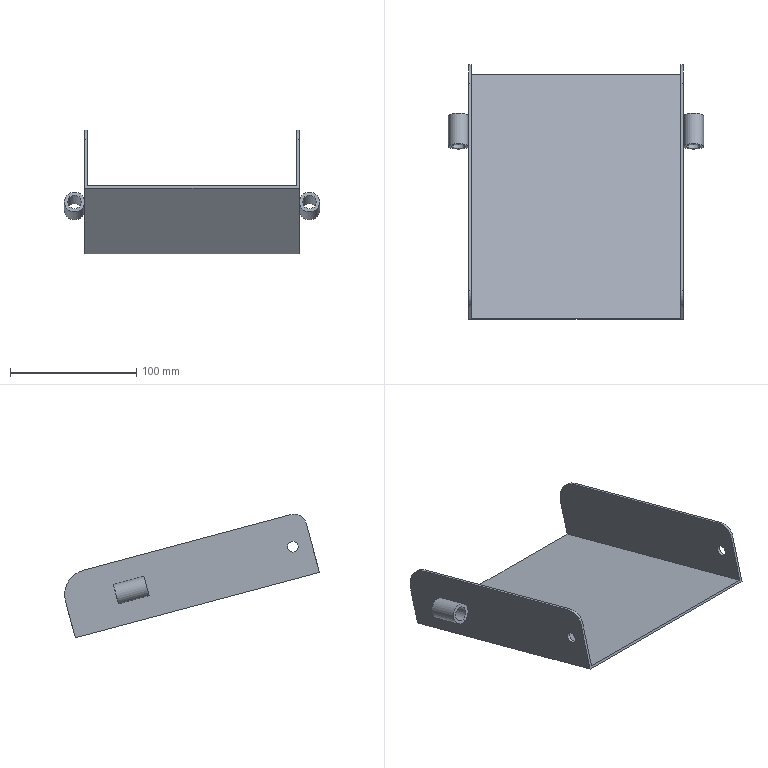Part | NX | features solid 2 | 1 solid | 28 faces | box 202 x 201.631 x 97.813 mm | volume 111062 mm3 | plane 18 | cylinder 10 | commonest cylinder face diameters 8.5 x2 11 x2 16 x2 20 x2 40 x2
STEP:
#1=CARTESIAN_POINT('',(-340.254,1380.577,-635.597));
#2=VERTEX_POINT('',#1);
#3=CARTESIAN_POINT('',(-340.,1380.577,-635.597));
#4=VERTEX_POINT('',#3);
#5=CARTESIAN_POINT('',(-342.,1380.577,-635.597));
#6=DIRECTION('',(1.,0.,0.));
#7=VECTOR('',#6,1000.);
#8=LINE('',#5,#7);
#9=EDGE_CURVE('',#2,#4,#8,.T.);
#10=ORIENTED_EDGE('',*,*,#9,.F.);
#11=CARTESIAN_POINT('',(-340.254,1356.429,-629.126));
#12=VERTEX_POINT('',#11);
#13=CARTESIAN_POINT('',(-340.254,1380.577,-635.597));
#14=DIRECTION('',(0.,-0.9659,0.2588));
#15=VECTOR('',#14,1000.);
#16=LINE('',#13,#15);
#17=EDGE_CURVE('',#2,#12,#16,.T.);
#18=ORIENTED_EDGE('',*,*,#17,.T.);
#19=CARTESIAN_POINT('',(-340.,1356.429,-629.126));
#20=VERTEX_POINT('',#19);
#21=CARTESIAN_POINT('',(-342.,1356.429,-629.126));
#22=DIRECTION('',(1.,0.,0.));
#23=VECTOR('',#22,1000.);
#24=LINE('',#21,#23);
#25=EDGE_CURVE('',#12,#20,#24,.T.);
#26=ORIENTED_EDGE('',*,*,#25,.T.);
#27=CARTESIAN_POINT('',(-340.,1226.029,-594.186));
#28=DIRECTION('',(0.,-0.9659,0.2588));
#29=VECTOR('',#28,1000.);
#30=LINE('',#27,#29);
#31=EDGE_CURVE('',#4,#20,#30,.T.);
#32=ORIENTED_EDGE('',*,*,#31,.F.);
#33=EDGE_LOOP('',(#10,#18,#26,#32));
#34=FACE_BOUND('',#33,.T.);
#35=CARTESIAN_POINT('',(-342.,1380.577,-635.597));
#36=DIRECTION('',(0.,0.2588,0.9659));
#37=DIRECTION('',(0.,-0.9659,0.2588));
#38=AXIS2_PLACEMENT_3D('',#35,#36,#37);
#39=PLANE('',#38);
#40=ADVANCED_FACE('',(#34),#39,.T.);
#41=CARTESIAN_POINT('',(-340.254,1379.542,-639.461));
#42=VERTEX_POINT('',#41);
#43=CARTESIAN_POINT('',(-340.254,1355.393,-632.99));
#44=VERTEX_POINT('',#43);
#45=CARTESIAN_POINT('',(-340.254,1379.542,-639.461));
#46=DIRECTION('',(0.,-0.9659,0.2588));
#47=VECTOR('',#46,1000.);
#48=LINE('',#45,#47);
#49=EDGE_CURVE('',#42,#44,#48,.T.);
#50=ORIENTED_EDGE('',*,*,#49,.F.);
#51=CARTESIAN_POINT('',(-340.,1379.542,-639.461));
#52=VERTEX_POINT('',#51);
#53=CARTESIAN_POINT('',(-342.,1379.542,-639.461));
#54=DIRECTION('',(1.,0.,0.));
#55=VECTOR('',#54,1000.);
#56=LINE('',#53,#55);
#57=EDGE_CURVE('',#42,#52,#56,.T.);
#58=ORIENTED_EDGE('',*,*,#57,.T.);
#59=CARTESIAN_POINT('',(-340.,1355.393,-632.99));
#60=VERTEX_POINT('',#59);
#61=CARTESIAN_POINT('',(-340.,1224.993,-598.05));
#62=DIRECTION('',(0.,-0.9659,0.2588));
#63=VECTOR('',#62,1000.);
#64=LINE('',#61,#63);
#65=EDGE_CURVE('',#52,#60,#64,.T.);
#66=ORIENTED_EDGE('',*,*,#65,.T.);
#67=CARTESIAN_POINT('',(-342.,1355.393,-632.99));
#68=DIRECTION('',(1.,0.,0.));
#69=VECTOR('',#68,1000.);
#70=LINE('',#67,#69);
#71=EDGE_CURVE('',#44,#60,#70,.T.);
#72=ORIENTED_EDGE('',*,*,#71,.F.);
#73=EDGE_LOOP('',(#50,#58,#66,#72));
#74=FACE_BOUND('',#73,.T.);
#75=CARTESIAN_POINT('',(-342.,1379.542,-639.461));
#76=DIRECTION('',(0.,0.2588,0.9659));
#77=DIRECTION('',(0.,-0.9659,0.2588));
#78=AXIS2_PLACEMENT_3D('',#75,#76,#77);
#79=PLANE('',#78);
#80=ADVANCED_FACE('',(#74),#79,.F.);
#81=CARTESIAN_POINT('',(-169.746,1380.577,-635.597));
#82=VERTEX_POINT('',#81);
#83=CARTESIAN_POINT('',(-169.746,1356.429,-629.126));
#84=VERTEX_POINT('',#83);
#85=CARTESIAN_POINT('',(-169.746,1380.577,-635.597));
#86=DIRECTION('',(0.,-0.9659,0.2588));
#87=VECTOR('',#86,1000.);
#88=LINE('',#85,#87);
#89=EDGE_CURVE('',#82,#84,#88,.T.);
#90=ORIENTED_EDGE('',*,*,#89,.F.);
#91=CARTESIAN_POINT('',(-170.,1380.577,-635.597));
#92=VERTEX_POINT('',#91);
#93=CARTESIAN_POINT('',(-168.,1380.577,-635.597));
#94=DIRECTION('',(1.,0.,0.));
#95=VECTOR('',#94,1000.);
#96=LINE('',#93,#95);
#97=EDGE_CURVE('',#82,#92,#96,.F.);
#98=ORIENTED_EDGE('',*,*,#97,.T.);
#99=CARTESIAN_POINT('',(-170.,1356.429,-629.126));
#100=VERTEX_POINT('',#99);
#101=CARTESIAN_POINT('',(-170.,1226.029,-594.186));
#102=DIRECTION('',(0.,0.9659,-0.2588));
#103=VECTOR('',#102,1000.);
#104=LINE('',#101,#103);
#105=EDGE_CURVE('',#92,#100,#104,.F.);
#106=ORIENTED_EDGE('',*,*,#105,.T.);
#107=CARTESIAN_POINT('',(-168.,1356.429,-629.126));
#108=DIRECTION('',(1.,0.,0.));
#109=VECTOR('',#108,1000.);
#110=LINE('',#107,#109);
#111=EDGE_CURVE('',#84,#100,#110,.F.);
#112=ORIENTED_EDGE('',*,*,#111,.F.);
#113=EDGE_LOOP('',(#90,#98,#106,#112));
#114=FACE_BOUND('',#113,.T.);
#115=CARTESIAN_POINT('',(-168.,1380.577,-635.597));
#116=DIRECTION('',(0.,-0.2588,-0.9659));
#117=DIRECTION('',(0.,0.9659,-0.2588));
#118=AXIS2_PLACEMENT_3D('',#115,#116,#117);
#119=PLANE('',#118);
#120=ADVANCED_FACE('',(#114),#119,.F.);
#121=CARTESIAN_POINT('',(-169.746,1379.542,-639.461));
#122=VERTEX_POINT('',#121);
#123=CARTESIAN_POINT('',(-170.,1379.542,-639.461));
#124=VERTEX_POINT('',#123);
#125=CARTESIAN_POINT('',(-168.,1379.542,-639.461));
#126=DIRECTION('',(1.,0.,0.));
#127=VECTOR('',#126,1000.);
#128=LINE('',#125,#127);
#129=EDGE_CURVE('',#122,#124,#128,.F.);
#130=ORIENTED_EDGE('',*,*,#129,.F.);
#131=CARTESIAN_POINT('',(-169.746,1355.393,-632.99));
#132=VERTEX_POINT('',#131);
#133=CARTESIAN_POINT('',(-169.746,1379.542,-639.461));
#134=DIRECTION('',(0.,-0.9659,0.2588));
#135=VECTOR('',#134,1000.);
#136=LINE('',#133,#135);
#137=EDGE_CURVE('',#122,#132,#136,.T.);
#138=ORIENTED_EDGE('',*,*,#137,.T.);
#139=CARTESIAN_POINT('',(-170.,1355.393,-632.99));
#140=VERTEX_POINT('',#139);
#141=CARTESIAN_POINT('',(-168.,1355.393,-632.99));
#142=DIRECTION('',(1.,0.,0.));
#143=VECTOR('',#142,1000.);
#144=LINE('',#141,#143);
#145=EDGE_CURVE('',#132,#140,#144,.F.);
#146=ORIENTED_EDGE('',*,*,#145,.T.);
#147=CARTESIAN_POINT('',(-170.,1224.993,-598.05));
#148=DIRECTION('',(0.,0.9659,-0.2588));
#149=VECTOR('',#148,1000.);
#150=LINE('',#147,#149);
#151=EDGE_CURVE('',#124,#140,#150,.F.);
#152=ORIENTED_EDGE('',*,*,#151,.F.);
#153=EDGE_LOOP('',(#130,#138,#146,#152));
#154=FACE_BOUND('',#153,.T.);
#155=CARTESIAN_POINT('',(-168.,1379.542,-639.461));
#156=DIRECTION('',(0.,-0.2588,-0.9659));
#157=DIRECTION('',(0.,0.9659,-0.2588));
#158=AXIS2_PLACEMENT_3D('',#155,#156,#157);
#159=PLANE('',#158);
#160=ADVANCED_FACE('',(#154),#159,.T.);
#161=CARTESIAN_POINT('',(-170.,1412.226,-672.03));
#162=VERTEX_POINT('',#161);
#163=CARTESIAN_POINT('',(-170.,1419.99,-643.052));
#164=VERTEX_POINT('',#163);
#165=CARTESIAN_POINT('',(-170.,1412.226,-672.03));
#166=DIRECTION('',(0.,-0.2588,-0.9659));
#167=VECTOR('',#166,1000.);
#168=LINE('',#165,#167);
#169=EDGE_CURVE('',#162,#164,#168,.F.);
#170=ORIENTED_EDGE('',*,*,#169,.T.);
#171=CARTESIAN_POINT('',(-170.,1405.848,-618.557));
#172=VERTEX_POINT('',#171);
#173=CARTESIAN_POINT('',(-170.,1400.672,-637.876));
#174=DIRECTION('',(-1.,0.,0.));
#175=DIRECTION('',(0.,-1.,0.));
#176=AXIS2_PLACEMENT_3D('',#173,#174,#175);
#177=CIRCLE('',#176,20.);
#178=EDGE_CURVE('',#172,#164,#177,.T.);
#179=ORIENTED_EDGE('',*,*,#178,.F.);
#180=CARTESIAN_POINT('',(-170.,1241.641,-574.558));
#181=VERTEX_POINT('',#180);
#182=CARTESIAN_POINT('',(-170.,1241.641,-574.558));
#183=DIRECTION('',(0.,0.9659,-0.2588));
#184=VECTOR('',#183,1000.);
#185=LINE('',#182,#184);
#186=EDGE_CURVE('',#181,#172,#185,.T.);
#187=ORIENTED_EDGE('',*,*,#186,.F.);
#188=CARTESIAN_POINT('',(-170.,1229.393,-581.629));
#189=VERTEX_POINT('',#188);
#190=CARTESIAN_POINT('',(-170.,1239.053,-584.217));
#191=DIRECTION('',(-1.,0.,0.));
#192=DIRECTION('',(0.,-1.,0.));
#193=AXIS2_PLACEMENT_3D('',#190,#191,#192);
#194=CIRCLE('',#193,10.);
#195=EDGE_CURVE('',#189,#181,#194,.T.);
#196=ORIENTED_EDGE('',*,*,#195,.F.);
#197=CARTESIAN_POINT('',(-170.,1219.041,-620.266));
#198=VERTEX_POINT('',#197);
#199=CARTESIAN_POINT('',(-170.,1219.041,-620.266));
#200=DIRECTION('',(0.,-0.2588,-0.9659));
#201=VECTOR('',#200,1000.);
#202=LINE('',#199,#201);
#203=EDGE_CURVE('',#198,#189,#202,.F.);
#204=ORIENTED_EDGE('',*,*,#203,.F.);
#205=CARTESIAN_POINT('',(-170.,1219.041,-620.266));
#206=DIRECTION('',(0.,0.9659,-0.2588));
#207=VECTOR('',#206,1000.);
#208=LINE('',#205,#207);
#209=EDGE_CURVE('',#198,#162,#208,.T.);
#210=ORIENTED_EDGE('',*,*,#209,.T.);
#211=EDGE_LOOP('',(#170,#179,#187,#196,#204,#210));
#212=FACE_BOUND('',#211,.T.);
#213=CARTESIAN_POINT('',(-170.,1240.,-595.75));
#214=VERTEX_POINT('',#213);
#215=CARTESIAN_POINT('',(-170.,1240.,-600.));
#216=DIRECTION('',(1.,0.,0.));
#217=DIRECTION('',(0.,0.,1.));
#218=AXIS2_PLACEMENT_3D('',#215,#216,#217);
#219=CIRCLE('',#218,4.25);
#220=EDGE_CURVE('',#214,#214,#219,.F.);
#221=ORIENTED_EDGE('',*,*,#220,.T.);
#222=EDGE_LOOP('',(#221));
#223=FACE_BOUND('',#222,.T.);
#224=ORIENTED_EDGE('',*,*,#105,.F.);
#225=CARTESIAN_POINT('',(-170.,1373.589,-661.677));
#226=DIRECTION('',(0.,-0.2588,-0.9659));
#227=VECTOR('',#226,1000.);
#228=LINE('',#225,#227);
#229=EDGE_CURVE('',#92,#124,#228,.T.);
#230=ORIENTED_EDGE('',*,*,#229,.T.);
#231=ORIENTED_EDGE('',*,*,#151,.T.);
#232=CARTESIAN_POINT('',(-170.,1349.441,-655.206));
#233=DIRECTION('',(0.,-0.2588,-0.9659));
#234=VECTOR('',#233,1000.);
#235=LINE('',#232,#234);
#236=EDGE_CURVE('',#140,#100,#235,.F.);
#237=ORIENTED_EDGE('',*,*,#236,.T.);
#238=EDGE_LOOP('',(#224,#230,#231,#237));
#239=FACE_BOUND('',#238,.T.);
#240=CARTESIAN_POINT('',(-170.,1219.041,-620.266));
#241=DIRECTION('',(1.,0.,0.));
#242=DIRECTION('',(0.,0.9659,-0.2588));
#243=AXIS2_PLACEMENT_3D('',#240,#241,#242);
#244=PLANE('',#243);
#245=ADVANCED_FACE('',(#212,#223,#239),#244,.T.);
#246=CARTESIAN_POINT('',(-172.,1412.743,-670.098));
#247=VERTEX_POINT('',#246);
#248=CARTESIAN_POINT('',(-338.,1412.743,-670.098));
#249=VERTEX_POINT('',#248);
#250=CARTESIAN_POINT('',(-170.,1412.743,-670.098));
#251=DIRECTION('',(1.,0.,0.));
#252=VECTOR('',#251,1000.);
#253=LINE('',#250,#252);
#254=EDGE_CURVE('',#247,#249,#253,.F.);
#255=ORIENTED_EDGE('',*,*,#254,.T.);
#256=CARTESIAN_POINT('',(-338.,1219.558,-618.334));
#257=VERTEX_POINT('',#256);
#258=CARTESIAN_POINT('',(-338.,1219.558,-618.334));
#259=DIRECTION('',(0.,-0.9659,0.2588));
#260=VECTOR('',#259,1000.);
#261=LINE('',#258,#260);
#262=EDGE_CURVE('',#249,#257,#261,.T.);
#263=ORIENTED_EDGE('',*,*,#262,.T.);
#264=CARTESIAN_POINT('',(-172.,1219.558,-618.334));
#265=VERTEX_POINT('',#264);
#266=CARTESIAN_POINT('',(-170.,1219.558,-618.334));
#267=DIRECTION('',(1.,0.,0.));
#268=VECTOR('',#267,1000.);
#269=LINE('',#266,#268);
#270=EDGE_CURVE('',#265,#257,#269,.F.);
#271=ORIENTED_EDGE('',*,*,#270,.F.);
#272=CARTESIAN_POINT('',(-172.,1219.558,-618.334));
#273=DIRECTION('',(0.,-0.9659,0.2588));
#274=VECTOR('',#273,1000.);
#275=LINE('',#272,#274);
#276=EDGE_CURVE('',#247,#265,#275,.T.);
#277=ORIENTED_EDGE('',*,*,#276,.F.);
#278=EDGE_LOOP('',(#255,#263,#271,#277));
#279=FACE_BOUND('',#278,.T.);
#280=CARTESIAN_POINT('',(-170.,1219.558,-618.334));
#281=DIRECTION('',(0.,0.2588,0.9659));
#282=DIRECTION('',(0.,-0.9659,0.2588));
#283=AXIS2_PLACEMENT_3D('',#280,#281,#282);
#284=PLANE('',#283);
#285=ADVANCED_FACE('',(#279),#284,.T.);
#286=CARTESIAN_POINT('',(-340.,1219.041,-620.266));
#287=VERTEX_POINT('',#286);
#288=CARTESIAN_POINT('',(-340.,1229.393,-581.629));
#289=VERTEX_POINT('',#288);
#290=CARTESIAN_POINT('',(-340.,1219.041,-620.266));
#291=DIRECTION('',(0.,-0.2588,-0.9659));
#292=VECTOR('',#291,1000.);
#293=LINE('',#290,#292);
#294=EDGE_CURVE('',#287,#289,#293,.F.);
#295=ORIENTED_EDGE('',*,*,#294,.F.);
#296=CARTESIAN_POINT('',(-170.,1219.041,-620.266));
#297=DIRECTION('',(-1.,0.,0.));
#298=VECTOR('',#297,1000.);
#299=LINE('',#296,#298);
#300=EDGE_CURVE('',#198,#287,#299,.T.);
#301=ORIENTED_EDGE('',*,*,#300,.F.);
#302=ORIENTED_EDGE('',*,*,#203,.T.);
#303=CARTESIAN_POINT('',(-172.,1229.393,-581.629));
#304=VERTEX_POINT('',#303);
#305=CARTESIAN_POINT('',(-172.,1229.393,-581.629));
#306=DIRECTION('',(1.,0.,0.));
#307=VECTOR('',#306,1000.);
#308=LINE('',#305,#307);
#309=EDGE_CURVE('',#304,#189,#308,.T.);
#310=ORIENTED_EDGE('',*,*,#309,.F.);
#311=CARTESIAN_POINT('',(-172.,1219.041,-620.266));
#312=DIRECTION('',(0.,0.2588,0.9659));
#313=VECTOR('',#312,1000.);
#314=LINE('',#311,#313);
#315=EDGE_CURVE('',#265,#304,#314,.T.);
#316=ORIENTED_EDGE('',*,*,#315,.F.);
#317=ORIENTED_EDGE('',*,*,#270,.T.);
#318=CARTESIAN_POINT('',(-338.,1229.393,-581.629));
#319=VERTEX_POINT('',#318);
#320=CARTESIAN_POINT('',(-338.,1219.041,-620.266));
#321=DIRECTION('',(0.,0.2588,0.9659));
#322=VECTOR('',#321,1000.);
#323=LINE('',#320,#322);
#324=EDGE_CURVE('',#257,#319,#323,.T.);
#325=ORIENTED_EDGE('',*,*,#324,.T.);
#326=CARTESIAN_POINT('',(-338.,1229.393,-581.629));
#327=DIRECTION('',(-1.,0.,0.));
#328=VECTOR('',#327,1000.);
#329=LINE('',#326,#328);
#330=EDGE_CURVE('',#319,#289,#329,.T.);
#331=ORIENTED_EDGE('',*,*,#330,.T.);
#332=EDGE_LOOP('',(#295,#301,#302,#310,#316,#317,#325,#331));
#333=FACE_BOUND('',#332,.T.);
#334=CARTESIAN_POINT('',(-170.,1219.041,-620.266));
#335=DIRECTION('',(0.,0.9659,-0.2588));
#336=DIRECTION('',(-1.,0.,0.));
#337=AXIS2_PLACEMENT_3D('',#334,#335,#336);
#338=PLANE('',#337);
#339=ADVANCED_FACE('',(#333),#338,.F.);
#340=CARTESIAN_POINT('',(-340.,1373.589,-661.677));
#341=DIRECTION('',(0.,-0.2588,-0.9659));
#342=VECTOR('',#341,1000.);
#343=LINE('',#340,#342);
#344=EDGE_CURVE('',#52,#4,#343,.F.);
#345=ORIENTED_EDGE('',*,*,#344,.T.);
#346=ORIENTED_EDGE('',*,*,#31,.T.);
#347=CARTESIAN_POINT('',(-340.,1349.441,-655.206));
#348=DIRECTION('',(0.,-0.2588,-0.9659));
#349=VECTOR('',#348,1000.);
#350=LINE('',#347,#349);
#351=EDGE_CURVE('',#20,#60,#350,.T.);
#352=ORIENTED_EDGE('',*,*,#351,.T.);
#353=ORIENTED_EDGE('',*,*,#65,.F.);
#354=EDGE_LOOP('',(#345,#346,#352,#353));
#355=FACE_BOUND('',#354,.T.);
#356=CARTESIAN_POINT('',(-340.,1240.,-595.75));
#357=VERTEX_POINT('',#356);
#358=CARTESIAN_POINT('',(-340.,1240.,-600.));
#359=DIRECTION('',(1.,0.,0.));
#360=DIRECTION('',(0.,0.,1.));
#361=AXIS2_PLACEMENT_3D('',#358,#359,#360);
#362=CIRCLE('',#361,4.25);
#363=EDGE_CURVE('',#357,#357,#362,.T.);
#364=ORIENTED_EDGE('',*,*,#363,.T.);
#365=EDGE_LOOP('',(#364));
#366=FACE_BOUND('',#365,.T.);
#367=ORIENTED_EDGE('',*,*,#294,.T.);
#368=CARTESIAN_POINT('',(-340.,1241.641,-574.558));
#369=VERTEX_POINT('',#368);
#370=CARTESIAN_POINT('',(-340.,1239.053,-584.217));
#371=DIRECTION('',(-1.,0.,0.));
#372=DIRECTION('',(0.,-1.,0.));
#373=AXIS2_PLACEMENT_3D('',#370,#371,#372);
#374=CIRCLE('',#373,10.);
#375=EDGE_CURVE('',#289,#369,#374,.T.);
#376=ORIENTED_EDGE('',*,*,#375,.T.);
#377=CARTESIAN_POINT('',(-340.,1405.848,-618.557));
#378=VERTEX_POINT('',#377);
#379=CARTESIAN_POINT('',(-340.,1241.641,-574.558));
#380=DIRECTION('',(0.,0.9659,-0.2588));
#381=VECTOR('',#380,1000.);
#382=LINE('',#379,#381);
#383=EDGE_CURVE('',#369,#378,#382,.T.);
#384=ORIENTED_EDGE('',*,*,#383,.T.);
#385=CARTESIAN_POINT('',(-340.,1419.99,-643.052));
#386=VERTEX_POINT('',#385);
#387=CARTESIAN_POINT('',(-340.,1400.672,-637.876));
#388=DIRECTION('',(-1.,0.,0.));
#389=DIRECTION('',(0.,-1.,0.));
#390=AXIS2_PLACEMENT_3D('',#387,#388,#389);
#391=CIRCLE('',#390,20.);
#392=EDGE_CURVE('',#378,#386,#391,.T.);
#393=ORIENTED_EDGE('',*,*,#392,.T.);
#394=CARTESIAN_POINT('',(-340.,1412.226,-672.03));
#395=VERTEX_POINT('',#394);
#396=CARTESIAN_POINT('',(-340.,1412.226,-672.03));
#397=DIRECTION('',(0.,-0.2588,-0.9659));
#398=VECTOR('',#397,1000.);
#399=LINE('',#396,#398);
#400=EDGE_CURVE('',#395,#386,#399,.F.);
#401=ORIENTED_EDGE('',*,*,#400,.F.);
#402=CARTESIAN_POINT('',(-340.,1219.041,-620.266));
#403=DIRECTION('',(0.,0.9659,-0.2588));
#404=VECTOR('',#403,1000.);
#405=LINE('',#402,#404);
#406=EDGE_CURVE('',#287,#395,#405,.T.);
#407=ORIENTED_EDGE('',*,*,#406,.F.);
#408=EDGE_LOOP('',(#367,#376,#384,#393,#401,#407));
#409=FACE_BOUND('',#408,.T.);
#410=CARTESIAN_POINT('',(-340.,1219.041,-620.266));
#411=DIRECTION('',(1.,0.,0.));
#412=DIRECTION('',(0.,0.9659,-0.2588));
#413=AXIS2_PLACEMENT_3D('',#410,#411,#412);
#414=PLANE('',#413);
#415=ADVANCED_FACE('',(#355,#366,#409),#414,.F.);
#416=ORIENTED_EDGE('',*,*,#400,.T.);
#417=CARTESIAN_POINT('',(-338.,1419.99,-643.052));
#418=VERTEX_POINT('',#417);
#419=CARTESIAN_POINT('',(-338.,1419.99,-643.052));
#420=DIRECTION('',(-1.,0.,0.));
#421=VECTOR('',#420,1000.);
#422=LINE('',#419,#421);
#423=EDGE_CURVE('',#418,#386,#422,.T.);
#424=ORIENTED_EDGE('',*,*,#423,.F.);
#425=CARTESIAN_POINT('',(-338.,1412.226,-672.03));
#426=DIRECTION('',(0.,0.2588,0.9659));
#427=VECTOR('',#426,1000.);
#428=LINE('',#425,#427);
#429=EDGE_CURVE('',#249,#418,#428,.T.);
#430=ORIENTED_EDGE('',*,*,#429,.F.);
#431=ORIENTED_EDGE('',*,*,#254,.F.);
#432=CARTESIAN_POINT('',(-172.,1419.99,-643.052));
#433=VERTEX_POINT('',#432);
#434=CARTESIAN_POINT('',(-172.,1412.226,-672.03));
#435=DIRECTION('',(0.,0.2588,0.9659));
#436=VECTOR('',#435,1000.);
#437=LINE('',#434,#436);
#438=EDGE_CURVE('',#247,#433,#437,.T.);
#439=ORIENTED_EDGE('',*,*,#438,.T.);
#440=CARTESIAN_POINT('',(-172.,1419.99,-643.052));
#441=DIRECTION('',(1.,0.,0.));
#442=VECTOR('',#441,1000.);
#443=LINE('',#440,#442);
#444=EDGE_CURVE('',#433,#164,#443,.T.);
#445=ORIENTED_EDGE('',*,*,#444,.T.);
#446=ORIENTED_EDGE('',*,*,#169,.F.);
#447=CARTESIAN_POINT('',(-170.,1412.226,-672.03));
#448=DIRECTION('',(-1.,0.,0.));
#449=VECTOR('',#448,1000.);
#450=LINE('',#447,#449);
#451=EDGE_CURVE('',#162,#395,#450,.T.);
#452=ORIENTED_EDGE('',*,*,#451,.T.);
#453=EDGE_LOOP('',(#416,#424,#430,#431,#439,#445,#446,#452));
#454=FACE_BOUND('',#453,.T.);
#455=CARTESIAN_POINT('',(-170.,1412.226,-672.03));
#456=DIRECTION('',(0.,0.9659,-0.2588));
#457=DIRECTION('',(-1.,0.,0.));
#458=AXIS2_PLACEMENT_3D('',#455,#456,#457);
#459=PLANE('',#458);
#460=ADVANCED_FACE('',(#454),#459,.T.);
#461=ORIENTED_EDGE('',*,*,#406,.T.);
#462=ORIENTED_EDGE('',*,*,#451,.F.);
#463=ORIENTED_EDGE('',*,*,#209,.F.);
#464=ORIENTED_EDGE('',*,*,#300,.T.);
#465=EDGE_LOOP('',(#461,#462,#463,#464));
#466=FACE_BOUND('',#465,.T.);
#467=CARTESIAN_POINT('',(-170.,1219.041,-620.266));
#468=DIRECTION('',(0.,0.2588,0.9659));
#469=DIRECTION('',(0.,-0.9659,0.2588));
#470=AXIS2_PLACEMENT_3D('',#467,#468,#469);
#471=PLANE('',#470);
#472=ADVANCED_FACE('',(#466),#471,.F.);
#473=ORIENTED_EDGE('',*,*,#178,.T.);
#474=ORIENTED_EDGE('',*,*,#444,.F.);
#475=CARTESIAN_POINT('',(-172.,1405.848,-618.557));
#476=VERTEX_POINT('',#475);
#477=CARTESIAN_POINT('',(-172.,1400.672,-637.876));
#478=DIRECTION('',(-1.,0.,0.));
#479=DIRECTION('',(0.,-1.,0.));
#480=AXIS2_PLACEMENT_3D('',#477,#478,#479);
#481=CIRCLE('',#480,20.);
#482=EDGE_CURVE('',#476,#433,#481,.T.);
#483=ORIENTED_EDGE('',*,*,#482,.F.);
#484=CARTESIAN_POINT('',(-172.,1405.848,-618.557));
#485=DIRECTION('',(1.,0.,0.));
#486=VECTOR('',#485,1000.);
#487=LINE('',#484,#486);
#488=EDGE_CURVE('',#476,#172,#487,.T.);
#489=ORIENTED_EDGE('',*,*,#488,.T.);
#490=EDGE_LOOP('',(#473,#474,#483,#489));
#491=FACE_BOUND('',#490,.T.);
#492=CARTESIAN_POINT('',(-172.,1400.672,-637.876));
#493=DIRECTION('',(1.,0.,0.));
#494=DIRECTION('',(0.,0.,1.));
#495=AXIS2_PLACEMENT_3D('',#492,#493,#494);
#496=CYLINDRICAL_SURFACE('',#495,20.);
#497=ADVANCED_FACE('',(#491),#496,.T.);
#498=ORIENTED_EDGE('',*,*,#195,.T.);
#499=CARTESIAN_POINT('',(-172.,1241.641,-574.558));
#500=VERTEX_POINT('',#499);
#501=CARTESIAN_POINT('',(-172.,1241.641,-574.558));
#502=DIRECTION('',(1.,0.,0.));
#503=VECTOR('',#502,1000.);
#504=LINE('',#501,#503);
#505=EDGE_CURVE('',#500,#181,#504,.T.);
#506=ORIENTED_EDGE('',*,*,#505,.F.);
#507=CARTESIAN_POINT('',(-172.,1239.053,-584.217));
#508=DIRECTION('',(-1.,0.,0.));
#509=DIRECTION('',(0.,-1.,0.));
#510=AXIS2_PLACEMENT_3D('',#507,#508,#509);
#511=CIRCLE('',#510,10.);
#512=EDGE_CURVE('',#304,#500,#511,.T.);
#513=ORIENTED_EDGE('',*,*,#512,.F.);
#514=ORIENTED_EDGE('',*,*,#309,.T.);
#515=EDGE_LOOP('',(#498,#506,#513,#514));
#516=FACE_BOUND('',#515,.T.);
#517=CARTESIAN_POINT('',(-172.,1239.053,-584.217));
#518=DIRECTION('',(1.,0.,0.));
#519=DIRECTION('',(0.,0.,1.));
#520=AXIS2_PLACEMENT_3D('',#517,#518,#519);
#521=CYLINDRICAL_SURFACE('',#520,10.);
#522=ADVANCED_FACE('',(#516),#521,.T.);
#523=ORIENTED_EDGE('',*,*,#186,.T.);
#524=ORIENTED_EDGE('',*,*,#488,.F.);
#525=CARTESIAN_POINT('',(-172.,1241.641,-574.558));
#526=DIRECTION('',(0.,0.9659,-0.2588));
#527=VECTOR('',#526,1000.);
#528=LINE('',#525,#527);
#529=EDGE_CURVE('',#500,#476,#528,.T.);
#530=ORIENTED_EDGE('',*,*,#529,.F.);
#531=ORIENTED_EDGE('',*,*,#505,.T.);
#532=EDGE_LOOP('',(#523,#524,#530,#531));
#533=FACE_BOUND('',#532,.T.);
#534=CARTESIAN_POINT('',(-172.,1241.641,-574.558));
#535=DIRECTION('',(0.,-0.2588,-0.9659));
#536=DIRECTION('',(0.,0.9659,-0.2588));
#537=AXIS2_PLACEMENT_3D('',#534,#535,#536);
#538=PLANE('',#537);
#539=ADVANCED_FACE('',(#533),#538,.F.);
#540=ORIENTED_EDGE('',*,*,#438,.F.);
#541=ORIENTED_EDGE('',*,*,#276,.T.);
#542=ORIENTED_EDGE('',*,*,#315,.T.);
#543=ORIENTED_EDGE('',*,*,#512,.T.);
#544=ORIENTED_EDGE('',*,*,#529,.T.);
#545=ORIENTED_EDGE('',*,*,#482,.T.);
#546=EDGE_LOOP('',(#540,#541,#542,#543,#544,#545));
#547=FACE_BOUND('',#546,.T.);
#548=CARTESIAN_POINT('',(-172.,1240.,-604.25));
#549=VERTEX_POINT('',#548);
#550=CARTESIAN_POINT('',(-172.,1240.,-600.));
#551=DIRECTION('',(-1.,0.,0.));
#552=DIRECTION('',(0.,0.,-1.));
#553=AXIS2_PLACEMENT_3D('',#550,#551,#552);
#554=CIRCLE('',#553,4.25);
#555=EDGE_CURVE('',#549,#549,#554,.T.);
#556=ORIENTED_EDGE('',*,*,#555,.F.);
#557=EDGE_LOOP('',(#556));
#558=FACE_BOUND('',#557,.T.);
#559=CARTESIAN_POINT('',(-172.,1400.672,-637.876));
#560=DIRECTION('',(-1.,0.,0.));
#561=DIRECTION('',(0.,0.,-1.));
#562=AXIS2_PLACEMENT_3D('',#559,#560,#561);
#563=PLANE('',#562);
#564=ADVANCED_FACE('',(#547,#558),#563,.T.);
#565=ORIENTED_EDGE('',*,*,#375,.F.);
#566=ORIENTED_EDGE('',*,*,#330,.F.);
#567=CARTESIAN_POINT('',(-338.,1241.641,-574.558));
#568=VERTEX_POINT('',#567);
#569=CARTESIAN_POINT('',(-338.,1239.053,-584.217));
#570=DIRECTION('',(-1.,0.,0.));
#571=DIRECTION('',(0.,-1.,0.));
#572=AXIS2_PLACEMENT_3D('',#569,#570,#571);
#573=CIRCLE('',#572,10.);
#574=EDGE_CURVE('',#319,#568,#573,.T.);
#575=ORIENTED_EDGE('',*,*,#574,.T.);
#576=CARTESIAN_POINT('',(-338.,1241.641,-574.558));
#577=DIRECTION('',(-1.,0.,0.));
#578=VECTOR('',#577,1000.);
#579=LINE('',#576,#578);
#580=EDGE_CURVE('',#568,#369,#579,.T.);
#581=ORIENTED_EDGE('',*,*,#580,.T.);
#582=EDGE_LOOP('',(#565,#566,#575,#581));
#583=FACE_BOUND('',#582,.T.);
#584=CARTESIAN_POINT('',(-338.,1239.053,-584.217));
#585=DIRECTION('',(-1.,0.,0.));
#586=DIRECTION('',(0.,0.,-1.));
#587=AXIS2_PLACEMENT_3D('',#584,#585,#586);
#588=CYLINDRICAL_SURFACE('',#587,10.);
#589=ADVANCED_FACE('',(#583),#588,.T.);
#590=ORIENTED_EDGE('',*,*,#383,.F.);
#591=ORIENTED_EDGE('',*,*,#580,.F.);
#592=CARTESIAN_POINT('',(-338.,1405.848,-618.557));
#593=VERTEX_POINT('',#592);
#594=CARTESIAN_POINT('',(-338.,1241.641,-574.558));
#595=DIRECTION('',(0.,0.9659,-0.2588));
#596=VECTOR('',#595,1000.);
#597=LINE('',#594,#596);
#598=EDGE_CURVE('',#568,#593,#597,.T.);
#599=ORIENTED_EDGE('',*,*,#598,.T.);
#600=CARTESIAN_POINT('',(-338.,1405.848,-618.557));
#601=DIRECTION('',(-1.,0.,0.));
#602=VECTOR('',#601,1000.);
#603=LINE('',#600,#602);
#604=EDGE_CURVE('',#593,#378,#603,.T.);
#605=ORIENTED_EDGE('',*,*,#604,.T.);
#606=EDGE_LOOP('',(#590,#591,#599,#605));
#607=FACE_BOUND('',#606,.T.);
#608=CARTESIAN_POINT('',(-338.,1241.641,-574.558));
#609=DIRECTION('',(0.,0.2588,0.9659));
#610=DIRECTION('',(0.,-0.9659,0.2588));
#611=AXIS2_PLACEMENT_3D('',#608,#609,#610);
#612=PLANE('',#611);
#613=ADVANCED_FACE('',(#607),#612,.T.);
#614=ORIENTED_EDGE('',*,*,#392,.F.);
#615=ORIENTED_EDGE('',*,*,#604,.F.);
#616=CARTESIAN_POINT('',(-338.,1400.672,-637.876));
#617=DIRECTION('',(-1.,0.,0.));
#618=DIRECTION('',(0.,-1.,0.));
#619=AXIS2_PLACEMENT_3D('',#616,#617,#618);
#620=CIRCLE('',#619,20.);
#621=EDGE_CURVE('',#593,#418,#620,.T.);
#622=ORIENTED_EDGE('',*,*,#621,.T.);
#623=ORIENTED_EDGE('',*,*,#423,.T.);
#624=EDGE_LOOP('',(#614,#615,#622,#623));
#625=FACE_BOUND('',#624,.T.);
#626=CARTESIAN_POINT('',(-338.,1400.672,-637.876));
#627=DIRECTION('',(-1.,0.,0.));
#628=DIRECTION('',(0.,0.,-1.));
#629=AXIS2_PLACEMENT_3D('',#626,#627,#628);
#630=CYLINDRICAL_SURFACE('',#629,20.);
#631=ADVANCED_FACE('',(#625),#630,.T.);
#632=CARTESIAN_POINT('',(-338.,1240.,-604.25));
#633=VERTEX_POINT('',#632);
#634=CARTESIAN_POINT('',(-338.,1240.,-600.));
#635=DIRECTION('',(-1.,0.,0.));
#636=DIRECTION('',(0.,0.,-1.));
#637=AXIS2_PLACEMENT_3D('',#634,#635,#636);
#638=CIRCLE('',#637,4.25);
#639=EDGE_CURVE('',#633,#633,#638,.T.);
#640=ORIENTED_EDGE('',*,*,#639,.T.);
#641=EDGE_LOOP('',(#640));
#642=FACE_BOUND('',#641,.T.);
#643=ORIENTED_EDGE('',*,*,#262,.F.);
#644=ORIENTED_EDGE('',*,*,#429,.T.);
#645=ORIENTED_EDGE('',*,*,#621,.F.);
#646=ORIENTED_EDGE('',*,*,#598,.F.);
#647=ORIENTED_EDGE('',*,*,#574,.F.);
#648=ORIENTED_EDGE('',*,*,#324,.F.);
#649=EDGE_LOOP('',(#643,#644,#645,#646,#647,#648));
#650=FACE_BOUND('',#649,.T.);
#651=CARTESIAN_POINT('',(-338.,1239.053,-584.217));
#652=DIRECTION('',(-1.,0.,0.));
#653=DIRECTION('',(0.,0.,-1.));
#654=AXIS2_PLACEMENT_3D('',#651,#652,#653);
#655=PLANE('',#654);
#656=ADVANCED_FACE('',(#642,#650),#655,.F.);
#657=ORIENTED_EDGE('',*,*,#639,.F.);
#658=EDGE_LOOP('',(#657));
#659=FACE_BOUND('',#658,.T.);
#660=ORIENTED_EDGE('',*,*,#363,.F.);
#661=EDGE_LOOP('',(#660));
#662=FACE_BOUND('',#661,.T.);
#663=CARTESIAN_POINT('',(145.,1240.,-600.));
#664=DIRECTION('',(-1.,0.,0.));
#665=DIRECTION('',(0.,0.,-1.));
#666=AXIS2_PLACEMENT_3D('',#663,#664,#665);
#667=CYLINDRICAL_SURFACE('',#666,4.25);
#668=ADVANCED_FACE('',(#659,#662),#667,.F.);
#669=ORIENTED_EDGE('',*,*,#555,.T.);
#670=EDGE_LOOP('',(#669));
#671=FACE_BOUND('',#670,.T.);
#672=ORIENTED_EDGE('',*,*,#220,.F.);
#673=EDGE_LOOP('',(#672));
#674=FACE_BOUND('',#673,.T.);
#675=CARTESIAN_POINT('',(145.,1240.,-600.));
#676=DIRECTION('',(-1.,0.,0.));
#677=DIRECTION('',(0.,0.,-1.));
#678=AXIS2_PLACEMENT_3D('',#675,#676,#677);
#679=CYLINDRICAL_SURFACE('',#678,4.25);
#680=ADVANCED_FACE('',(#671,#674),#679,.F.);
#681=ORIENTED_EDGE('',*,*,#129,.T.);
#682=ORIENTED_EDGE('',*,*,#229,.F.);
#683=ORIENTED_EDGE('',*,*,#97,.F.);
#684=CARTESIAN_POINT('',(-162.,1380.059,-637.529));
#685=DIRECTION('',(0.,0.9659,-0.2588));
#686=DIRECTION('',(0.,0.2588,0.9659));
#687=AXIS2_PLACEMENT_3D('',#684,#685,#686);
#688=CIRCLE('',#687,8.);
#689=EDGE_CURVE('',#82,#122,#688,.T.);
#690=ORIENTED_EDGE('',*,*,#689,.T.);
#691=EDGE_LOOP('',(#681,#682,#683,#690));
#692=FACE_BOUND('',#691,.T.);
#693=CARTESIAN_POINT('',(-162.,1381.483,-632.216));
#694=VERTEX_POINT('',#693);
#695=CARTESIAN_POINT('',(-162.,1380.059,-637.529));
#696=DIRECTION('',(0.,0.9659,-0.2588));
#697=DIRECTION('',(0.,0.2588,0.9659));
#698=AXIS2_PLACEMENT_3D('',#695,#696,#697);
#699=CIRCLE('',#698,5.5);
#700=EDGE_CURVE('',#694,#694,#699,.T.);
#701=ORIENTED_EDGE('',*,*,#700,.F.);
#702=EDGE_LOOP('',(#701));
#703=FACE_BOUND('',#702,.T.);
#704=CARTESIAN_POINT('',(-168.,1380.059,-637.529));
#705=DIRECTION('',(0.,-0.9659,0.2588));
#706=DIRECTION('',(-1.,0.,0.));
#707=AXIS2_PLACEMENT_3D('',#704,#705,#706);
#708=PLANE('',#707);
#709=ADVANCED_FACE('',(#692,#703),#708,.F.);
#710=CARTESIAN_POINT('',(-162.,1355.911,-631.058));
#711=DIRECTION('',(0.,-0.9659,0.2588));
#712=DIRECTION('',(0.,-0.2588,-0.9659));
#713=AXIS2_PLACEMENT_3D('',#710,#711,#712);
#714=CIRCLE('',#713,8.);
#715=EDGE_CURVE('',#132,#84,#714,.T.);
#716=ORIENTED_EDGE('',*,*,#715,.T.);
#717=ORIENTED_EDGE('',*,*,#111,.T.);
#718=ORIENTED_EDGE('',*,*,#236,.F.);
#719=ORIENTED_EDGE('',*,*,#145,.F.);
#720=EDGE_LOOP('',(#716,#717,#718,#719));
#721=FACE_BOUND('',#720,.T.);
#722=CARTESIAN_POINT('',(-162.,1354.488,-636.371));
#723=VERTEX_POINT('',#722);
#724=CARTESIAN_POINT('',(-162.,1355.911,-631.058));
#725=DIRECTION('',(0.,-0.9659,0.2588));
#726=DIRECTION('',(0.,-0.2588,-0.9659));
#727=AXIS2_PLACEMENT_3D('',#724,#725,#726);
#728=CIRCLE('',#727,5.5);
#729=EDGE_CURVE('',#723,#723,#728,.T.);
#730=ORIENTED_EDGE('',*,*,#729,.F.);
#731=EDGE_LOOP('',(#730));
#732=FACE_BOUND('',#731,.T.);
#733=CARTESIAN_POINT('',(-168.,1355.911,-631.058));
#734=DIRECTION('',(0.,-0.9659,0.2588));
#735=DIRECTION('',(-1.,0.,0.));
#736=AXIS2_PLACEMENT_3D('',#733,#734,#735);
#737=PLANE('',#736);
#738=ADVANCED_FACE('',(#721,#732),#737,.T.);
#739=ORIENTED_EDGE('',*,*,#689,.F.);
#740=ORIENTED_EDGE('',*,*,#89,.T.);
#741=ORIENTED_EDGE('',*,*,#715,.F.);
#742=ORIENTED_EDGE('',*,*,#137,.F.);
#743=EDGE_LOOP('',(#739,#740,#741,#742));
#744=FACE_BOUND('',#743,.T.);
#745=CARTESIAN_POINT('',(-162.,1380.059,-637.529));
#746=DIRECTION('',(0.,-0.9659,0.2588));
#747=DIRECTION('',(0.,-0.2588,-0.9659));
#748=AXIS2_PLACEMENT_3D('',#745,#746,#747);
#749=CYLINDRICAL_SURFACE('',#748,8.);
#750=ADVANCED_FACE('',(#744),#749,.T.);
#751=ORIENTED_EDGE('',*,*,#700,.T.);
#752=EDGE_LOOP('',(#751));
#753=FACE_BOUND('',#752,.T.);
#754=ORIENTED_EDGE('',*,*,#729,.T.);
#755=EDGE_LOOP('',(#754));
#756=FACE_BOUND('',#755,.T.);
#757=CARTESIAN_POINT('',(-162.,1380.059,-637.529));
#758=DIRECTION('',(0.,-0.9659,0.2588));
#759=DIRECTION('',(0.,-0.2588,-0.9659));
#760=AXIS2_PLACEMENT_3D('',#757,#758,#759);
#761=CYLINDRICAL_SURFACE('',#760,5.5);
#762=ADVANCED_FACE('',(#753,#756),#761,.F.);
#763=ORIENTED_EDGE('',*,*,#71,.T.);
#764=ORIENTED_EDGE('',*,*,#351,.F.);
#765=ORIENTED_EDGE('',*,*,#25,.F.);
#766=CARTESIAN_POINT('',(-348.,1355.911,-631.058));
#767=DIRECTION('',(0.,-0.9659,0.2588));
#768=DIRECTION('',(0.,-0.2588,-0.9659));
#769=AXIS2_PLACEMENT_3D('',#766,#767,#768);
#770=CIRCLE('',#769,8.);
#771=EDGE_CURVE('',#12,#44,#770,.T.);
#772=ORIENTED_EDGE('',*,*,#771,.T.);
#773=EDGE_LOOP('',(#763,#764,#765,#772));
#774=FACE_BOUND('',#773,.T.);
#775=CARTESIAN_POINT('',(-348.,1354.488,-636.371));
#776=VERTEX_POINT('',#775);
#777=CARTESIAN_POINT('',(-348.,1355.911,-631.058));
#778=DIRECTION('',(0.,-0.9659,0.2588));
#779=DIRECTION('',(0.,-0.2588,-0.9659));
#780=AXIS2_PLACEMENT_3D('',#777,#778,#779);
#781=CIRCLE('',#780,5.5);
#782=EDGE_CURVE('',#776,#776,#781,.T.);
#783=ORIENTED_EDGE('',*,*,#782,.F.);
#784=EDGE_LOOP('',(#783));
#785=FACE_BOUND('',#784,.T.);
#786=CARTESIAN_POINT('',(-342.,1355.911,-631.058));
#787=DIRECTION('',(0.,-0.9659,0.2588));
#788=DIRECTION('',(1.,0.,0.));
#789=AXIS2_PLACEMENT_3D('',#786,#787,#788);
#790=PLANE('',#789);
#791=ADVANCED_FACE('',(#774,#785),#790,.T.);
#792=CARTESIAN_POINT('',(-348.,1380.059,-637.529));
#793=DIRECTION('',(0.,0.9659,-0.2588));
#794=DIRECTION('',(0.,0.2588,0.9659));
#795=AXIS2_PLACEMENT_3D('',#792,#793,#794);
#796=CIRCLE('',#795,8.);
#797=EDGE_CURVE('',#42,#2,#796,.T.);
#798=ORIENTED_EDGE('',*,*,#797,.T.);
#799=ORIENTED_EDGE('',*,*,#9,.T.);
#800=ORIENTED_EDGE('',*,*,#344,.F.);
#801=ORIENTED_EDGE('',*,*,#57,.F.);
#802=EDGE_LOOP('',(#798,#799,#800,#801));
#803=FACE_BOUND('',#802,.T.);
#804=CARTESIAN_POINT('',(-348.,1381.483,-632.216));
#805=VERTEX_POINT('',#804);
#806=CARTESIAN_POINT('',(-348.,1380.059,-637.529));
#807=DIRECTION('',(0.,0.9659,-0.2588));
#808=DIRECTION('',(0.,0.2588,0.9659));
#809=AXIS2_PLACEMENT_3D('',#806,#807,#808);
#810=CIRCLE('',#809,5.5);
#811=EDGE_CURVE('',#805,#805,#810,.T.);
#812=ORIENTED_EDGE('',*,*,#811,.F.);
#813=EDGE_LOOP('',(#812));
#814=FACE_BOUND('',#813,.T.);
#815=CARTESIAN_POINT('',(-342.,1380.059,-637.529));
#816=DIRECTION('',(0.,-0.9659,0.2588));
#817=DIRECTION('',(1.,0.,0.));
#818=AXIS2_PLACEMENT_3D('',#815,#816,#817);
#819=PLANE('',#818);
#820=ADVANCED_FACE('',(#803,#814),#819,.F.);
#821=ORIENTED_EDGE('',*,*,#17,.F.);
#822=ORIENTED_EDGE('',*,*,#797,.F.);
#823=ORIENTED_EDGE('',*,*,#49,.T.);
#824=ORIENTED_EDGE('',*,*,#771,.F.);
#825=EDGE_LOOP('',(#821,#822,#823,#824));
#826=FACE_BOUND('',#825,.T.);
#827=CARTESIAN_POINT('',(-348.,1380.059,-637.529));
#828=DIRECTION('',(0.,-0.9659,0.2588));
#829=DIRECTION('',(0.,-0.2588,-0.9659));
#830=AXIS2_PLACEMENT_3D('',#827,#828,#829);
#831=CYLINDRICAL_SURFACE('',#830,8.);
#832=ADVANCED_FACE('',(#826),#831,.T.);
#833=ORIENTED_EDGE('',*,*,#811,.T.);
#834=EDGE_LOOP('',(#833));
#835=FACE_BOUND('',#834,.T.);
#836=ORIENTED_EDGE('',*,*,#782,.T.);
#837=EDGE_LOOP('',(#836));
#838=FACE_BOUND('',#837,.T.);
#839=CARTESIAN_POINT('',(-348.,1380.059,-637.529));
#840=DIRECTION('',(0.,-0.9659,0.2588));
#841=DIRECTION('',(0.,-0.2588,-0.9659));
#842=AXIS2_PLACEMENT_3D('',#839,#840,#841);
#843=CYLINDRICAL_SURFACE('',#842,5.5);
#844=ADVANCED_FACE('',(#835,#838),#843,.F.);
#845=CLOSED_SHELL('',(#40,#80,#120,#160,#245,#285,#339,#415,#460,#472,#497,#522,#539,#564,#589,#613,#631,#656,#668,#680,#709,#738,#750,#762,#791,#820,#832,#844));
#846=MANIFOLD_SOLID_BREP('',#845);
#847=(LENGTH_UNIT()NAMED_UNIT(*)SI_UNIT(.MILLI.,.METRE.));
#848=UNCERTAINTY_MEASURE_WITH_UNIT(LENGTH_MEASURE(0.00001),#847,'','');
#849=(NAMED_UNIT(*)PLANE_ANGLE_UNIT()SI_UNIT($,.RADIAN.));
#850=(NAMED_UNIT(*)SI_UNIT($,.STERADIAN.)SOLID_ANGLE_UNIT());
#851=(GEOMETRIC_REPRESENTATION_CONTEXT(3)GLOBAL_UNCERTAINTY_ASSIGNED_CONTEXT((#848))GLOBAL_UNIT_ASSIGNED_CONTEXT((#847,#849,#850))REPRESENTATION_CONTEXT('',''));
#852=ADVANCED_BREP_SHAPE_REPRESENTATION('',(#846),#851);